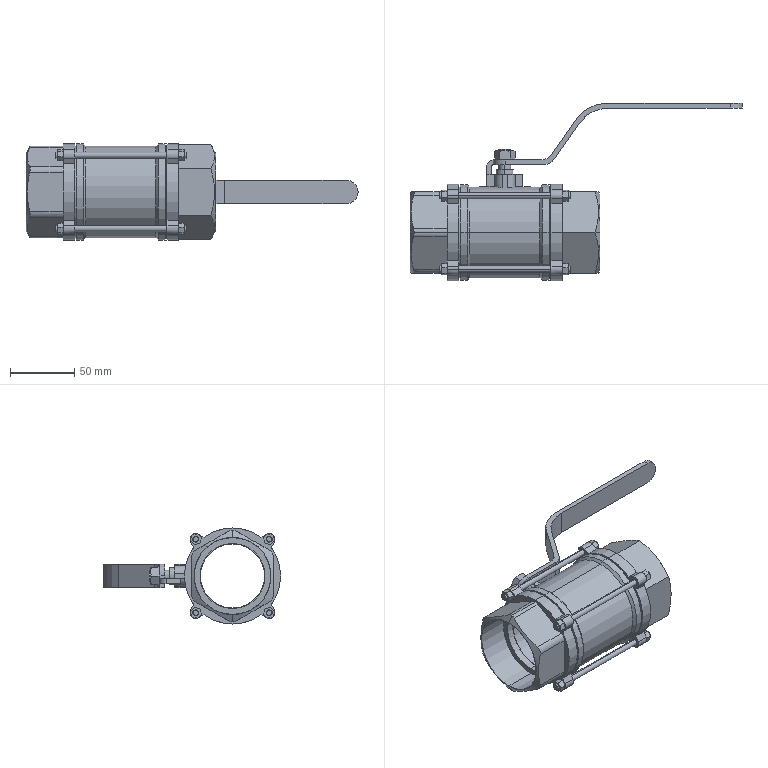Part | SolidWorks | features Boss 8, Fillet 5, MirrorPattern 3, RevCut 2, Revolution 2, Chamfer 1, CirPattern 1, Cut 1, ICE 1 | 2 solids | 287 faces | box 259 x 138.2 x 75 mm | volume 272305 mm3 | plane 157 | cylinder 92 | cone 38 | commonest cylinder face diameters 4.725 x24 75 x14 8.958 x12 12.192 x7 18.5 x5 9.324 x4